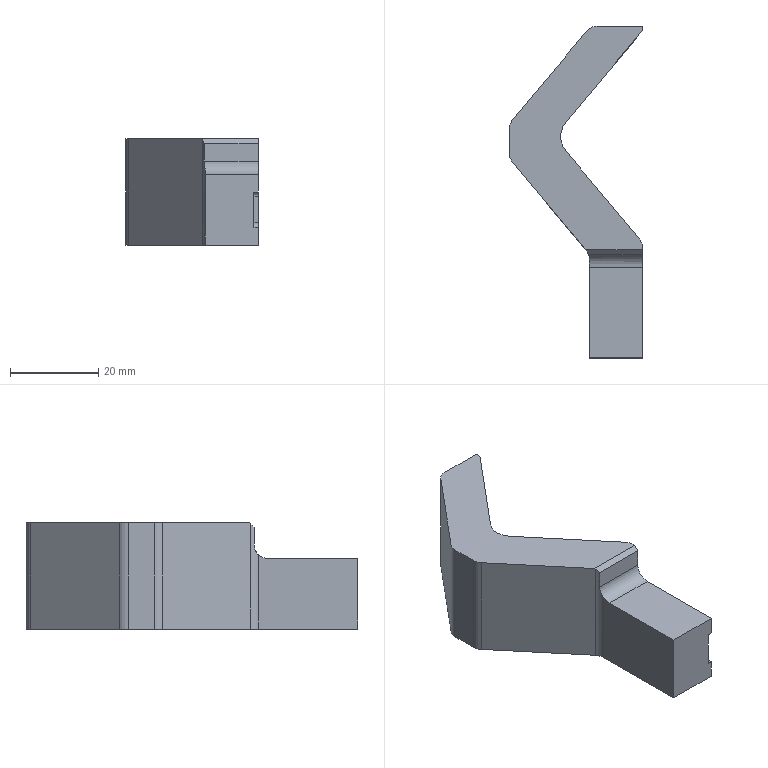Part | STEP file | 001-010-Waste gripper | 1 solid | 28 faces | box 30 x 75 x 24 mm | volume 20563 mm3 | plane 19 | cylinder 9 | commonest cylinder face diameters 6 x6 2 x2 10 x1